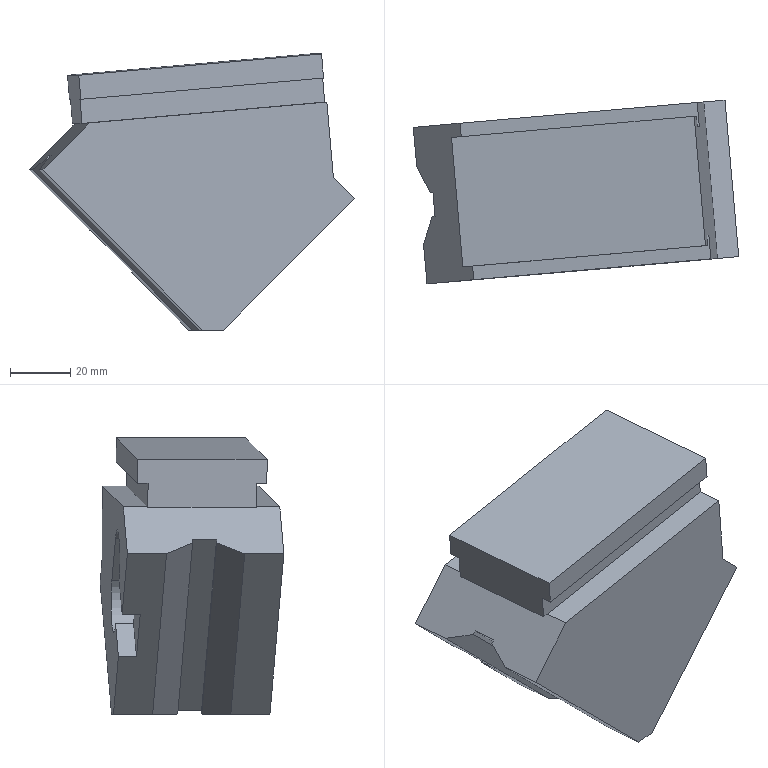Part | NX | features solid 2 | 1 solid | 35 faces | box 107.729 x 60.831 x 91.402 mm | volume 279477 mm3 | plane 33 | cylinder 2 | commonest cylinder face diameters 20 x2
STEP:
#1=CARTESIAN_POINT('',(-444.721,27.344,108.351));
#2=VERTEX_POINT('',#1);
#3=CARTESIAN_POINT('',(-445.418,35.314,108.351));
#4=VERTEX_POINT('',#3);
#5=CARTESIAN_POINT('',(-440.886,-16.489,108.351));
#6=DIRECTION('',(-0.08716,0.9962,0.));
#7=VECTOR('',#6,1000.);
#8=LINE('',#5,#7);
#9=EDGE_CURVE('',#2,#4,#8,.T.);
#10=ORIENTED_EDGE('',*,*,#9,.F.);
#11=CARTESIAN_POINT('',(-366.215,34.212,115.246));
#12=VERTEX_POINT('',#11);
#13=CARTESIAN_POINT('',(-440.646,27.701,108.709));
#14=DIRECTION('',(0.9924,0.08682,0.08716));
#15=VECTOR('',#14,1000.);
#16=LINE('',#13,#15);
#17=EDGE_CURVE('',#2,#12,#16,.T.);
#18=ORIENTED_EDGE('',*,*,#17,.T.);
#19=CARTESIAN_POINT('',(-366.913,42.182,115.246));
#20=VERTEX_POINT('',#19);
#21=CARTESIAN_POINT('',(-362.38,-9.62,115.246));
#22=DIRECTION('',(-0.08716,0.9962,0.));
#23=VECTOR('',#22,1000.);
#24=LINE('',#21,#23);
#25=EDGE_CURVE('',#12,#20,#24,.T.);
#26=ORIENTED_EDGE('',*,*,#25,.T.);
#27=CARTESIAN_POINT('',(-445.418,35.314,108.351));
#28=DIRECTION('',(0.9924,0.08682,0.08716));
#29=VECTOR('',#28,1000.);
#30=LINE('',#27,#29);
#31=EDGE_CURVE('',#4,#20,#30,.T.);
#32=ORIENTED_EDGE('',*,*,#31,.F.);
#33=EDGE_LOOP('',(#10,#18,#26,#32));
#34=FACE_BOUND('',#33,.T.);
#35=CARTESIAN_POINT('',(-440.886,-16.489,108.351));
#36=DIRECTION('',(-0.08682,-0.007596,0.9962));
#37=DIRECTION('',(0.9924,0.08682,0.08716));
#38=AXIS2_PLACEMENT_3D('',#35,#36,#37);
#39=PLANE('',#38);
#40=ADVANCED_FACE('',(#34),#39,.T.);
#41=CARTESIAN_POINT('',(-415.583,31.901,69.751));
#42=VERTEX_POINT('',#41);
#43=CARTESIAN_POINT('',(-415.06,25.924,69.751));
#44=VERTEX_POINT('',#43);
#45=CARTESIAN_POINT('',(-415.06,25.924,69.751));
#46=DIRECTION('',(0.08716,-0.9962,0.));
#47=VECTOR('',#46,1000.);
#48=LINE('',#45,#47);
#49=EDGE_CURVE('',#42,#44,#48,.T.);
#50=ORIENTED_EDGE('',*,*,#49,.F.);
#51=CARTESIAN_POINT('',(-429.629,30.672,83.85));
#52=VERTEX_POINT('',#51);
#53=CARTESIAN_POINT('',(-415.541,31.905,69.708));
#54=DIRECTION('',(-0.7044,-0.06163,0.7071));
#55=VECTOR('',#54,1000.);
#56=LINE('',#53,#55);
#57=EDGE_CURVE('',#42,#52,#56,.T.);
#58=ORIENTED_EDGE('',*,*,#57,.T.);
#59=CARTESIAN_POINT('',(-429.106,24.695,83.85));
#60=VERTEX_POINT('',#59);
#61=CARTESIAN_POINT('',(-429.106,24.695,83.85));
#62=DIRECTION('',(-0.08716,0.9962,0.));
#63=VECTOR('',#62,1000.);
#64=LINE('',#61,#63);
#65=EDGE_CURVE('',#60,#52,#64,.T.);
#66=ORIENTED_EDGE('',*,*,#65,.F.);
#67=CARTESIAN_POINT('',(-415.018,25.927,69.708));
#68=DIRECTION('',(-0.7044,-0.06163,0.7071));
#69=VECTOR('',#68,1000.);
#70=LINE('',#67,#69);
#71=EDGE_CURVE('',#44,#60,#70,.T.);
#72=ORIENTED_EDGE('',*,*,#71,.F.);
#73=EDGE_LOOP('',(#50,#58,#66,#72));
#74=FACE_BOUND('',#73,.T.);
#75=CARTESIAN_POINT('',(-415.018,25.927,69.708));
#76=DIRECTION('',(-0.7044,-0.06163,-0.7071));
#77=DIRECTION('',(-0.7044,-0.06163,0.7071));
#78=AXIS2_PLACEMENT_3D('',#75,#76,#77);
#79=PLANE('',#78);
#80=ADVANCED_FACE('',(#74),#79,.F.);
#81=CARTESIAN_POINT('',(-402.018,39.111,83.893));
#82=VERTEX_POINT('',#81);
#83=CARTESIAN_POINT('',(-416.064,37.882,97.992));
#84=VERTEX_POINT('',#83);
#85=CARTESIAN_POINT('',(-401.976,39.114,83.85));
#86=DIRECTION('',(-0.7044,-0.06163,0.7071));
#87=VECTOR('',#86,1000.);
#88=LINE('',#85,#87);
#89=EDGE_CURVE('',#82,#84,#88,.T.);
#90=ORIENTED_EDGE('',*,*,#89,.F.);
#91=CARTESIAN_POINT('',(-400.972,27.156,83.893));
#92=VERTEX_POINT('',#91);
#93=CARTESIAN_POINT('',(-400.972,27.156,83.893));
#94=DIRECTION('',(-0.08716,0.9962,0.));
#95=VECTOR('',#94,1000.);
#96=LINE('',#93,#95);
#97=EDGE_CURVE('',#92,#82,#96,.T.);
#98=ORIENTED_EDGE('',*,*,#97,.F.);
#99=CARTESIAN_POINT('',(-415.018,25.927,97.992));
#100=VERTEX_POINT('',#99);
#101=CARTESIAN_POINT('',(-400.93,27.16,83.85));
#102=DIRECTION('',(-0.7044,-0.06163,0.7071));
#103=VECTOR('',#102,1000.);
#104=LINE('',#101,#103);
#105=EDGE_CURVE('',#92,#100,#104,.T.);
#106=ORIENTED_EDGE('',*,*,#105,.T.);
#107=CARTESIAN_POINT('',(-415.018,25.927,97.992));
#108=DIRECTION('',(-0.08716,0.9962,0.));
#109=VECTOR('',#108,1000.);
#110=LINE('',#107,#109);
#111=EDGE_CURVE('',#100,#84,#110,.T.);
#112=ORIENTED_EDGE('',*,*,#111,.T.);
#113=EDGE_LOOP('',(#90,#98,#106,#112));
#114=FACE_BOUND('',#113,.T.);
#115=CARTESIAN_POINT('',(-400.93,27.16,83.85));
#116=DIRECTION('',(-0.7044,-0.06163,-0.7071));
#117=DIRECTION('',(-0.7044,-0.06163,0.7071));
#118=AXIS2_PLACEMENT_3D('',#115,#116,#117);
#119=PLANE('',#118);
#120=ADVANCED_FACE('',(#114),#119,.T.);
#121=CARTESIAN_POINT('',(-357.698,42.988,83.27));
#122=VERTEX_POINT('',#121);
#123=CARTESIAN_POINT('',(-401.019,39.198,39.783));
#124=VERTEX_POINT('',#123);
#125=CARTESIAN_POINT('',(-357.698,42.988,83.27));
#126=DIRECTION('',(-0.7044,-0.06163,-0.7071));
#127=VECTOR('',#126,1000.);
#128=LINE('',#125,#127);
#129=EDGE_CURVE('',#122,#124,#128,.T.);
#130=ORIENTED_EDGE('',*,*,#129,.T.);
#131=CARTESIAN_POINT('',(-408.064,38.582,39.783));
#132=VERTEX_POINT('',#131);
#133=CARTESIAN_POINT('',(-401.019,39.198,39.783));
#134=DIRECTION('',(-0.9962,-0.08716,0.));
#135=VECTOR('',#134,1000.);
#136=LINE('',#133,#135);
#137=EDGE_CURVE('',#124,#132,#136,.T.);
#138=ORIENTED_EDGE('',*,*,#137,.T.);
#139=CARTESIAN_POINT('',(-426.969,36.928,58.761));
#140=VERTEX_POINT('',#139);
#141=CARTESIAN_POINT('',(-460.895,33.96,92.816));
#142=DIRECTION('',(0.7044,0.06163,-0.7071));
#143=VECTOR('',#142,1000.);
#144=LINE('',#141,#143);
#145=EDGE_CURVE('',#140,#132,#144,.T.);
#146=ORIENTED_EDGE('',*,*,#145,.F.);
#147=CARTESIAN_POINT('',(-416.064,37.882,69.708));
#148=VERTEX_POINT('',#147);
#149=CARTESIAN_POINT('',(-401.976,39.114,83.85));
#150=DIRECTION('',(-0.7044,-0.06163,-0.7071));
#151=VECTOR('',#150,1000.);
#152=LINE('',#149,#151);
#153=EDGE_CURVE('',#148,#140,#152,.T.);
#154=ORIENTED_EDGE('',*,*,#153,.F.);
#155=CARTESIAN_POINT('',(-416.106,37.878,69.751));
#156=VERTEX_POINT('',#155);
#157=CARTESIAN_POINT('',(-416.106,37.878,69.751));
#158=DIRECTION('',(0.7044,0.06163,-0.7071));
#159=VECTOR('',#158,1000.);
#160=LINE('',#157,#159);
#161=EDGE_CURVE('',#156,#148,#160,.T.);
#162=ORIENTED_EDGE('',*,*,#161,.F.);
#163=CARTESIAN_POINT('',(-409.062,38.494,76.822));
#164=DIRECTION('',(0.08716,-0.9962,0.));
#165=DIRECTION('',(0.9029,0.07899,-0.4226));
#166=AXIS2_PLACEMENT_3D('',#163,#164,#165);
#167=CIRCLE('',#166,10.);
#168=EDGE_CURVE('',#156,#82,#167,.T.);
#169=ORIENTED_EDGE('',*,*,#168,.T.);
#170=ORIENTED_EDGE('',*,*,#89,.T.);
#171=CARTESIAN_POINT('',(-430.152,36.649,83.85));
#172=VERTEX_POINT('',#171);
#173=CARTESIAN_POINT('',(-423.108,37.266,90.921));
#174=DIRECTION('',(0.08716,-0.9962,0.));
#175=DIRECTION('',(0.9029,0.07899,-0.4226));
#176=AXIS2_PLACEMENT_3D('',#173,#174,#175);
#177=CIRCLE('',#176,10.);
#178=EDGE_CURVE('',#84,#172,#177,.T.);
#179=ORIENTED_EDGE('',*,*,#178,.T.);
#180=CARTESIAN_POINT('',(-441.058,35.695,72.903));
#181=VERTEX_POINT('',#180);
#182=CARTESIAN_POINT('',(-416.064,37.882,97.992));
#183=DIRECTION('',(-0.7044,-0.06163,-0.7071));
#184=VECTOR('',#183,1000.);
#185=LINE('',#182,#184);
#186=EDGE_CURVE('',#172,#181,#185,.T.);
#187=ORIENTED_EDGE('',*,*,#186,.T.);
#188=CARTESIAN_POINT('',(-460.895,33.96,92.816));
#189=VERTEX_POINT('',#188);
#190=CARTESIAN_POINT('',(-460.895,33.96,92.816));
#191=DIRECTION('',(0.7044,0.06163,-0.7071));
#192=VECTOR('',#191,1000.);
#193=LINE('',#190,#192);
#194=EDGE_CURVE('',#189,#181,#193,.T.);
#195=ORIENTED_EDGE('',*,*,#194,.F.);
#196=CARTESIAN_POINT('',(-445.418,35.314,108.351));
#197=DIRECTION('',(-0.7044,-0.06163,-0.7071));
#198=VECTOR('',#197,1000.);
#199=LINE('',#196,#198);
#200=EDGE_CURVE('',#4,#189,#199,.T.);
#201=ORIENTED_EDGE('',*,*,#200,.F.);
#202=ORIENTED_EDGE('',*,*,#31,.T.);
#203=CARTESIAN_POINT('',(-364.742,42.372,90.341));
#204=VERTEX_POINT('',#203);
#205=CARTESIAN_POINT('',(-366.913,42.182,115.246));
#206=DIRECTION('',(0.08682,0.007596,-0.9962));
#207=VECTOR('',#206,1000.);
#208=LINE('',#205,#207);
#209=EDGE_CURVE('',#20,#204,#208,.T.);
#210=ORIENTED_EDGE('',*,*,#209,.T.);
#211=CARTESIAN_POINT('',(-364.742,42.372,90.341));
#212=DIRECTION('',(0.7044,0.06163,-0.7071));
#213=VECTOR('',#212,1000.);
#214=LINE('',#211,#213);
#215=EDGE_CURVE('',#204,#122,#214,.T.);
#216=ORIENTED_EDGE('',*,*,#215,.T.);
#217=EDGE_LOOP('',(#130,#138,#146,#154,#162,#169,#170,#179,#187,#195,#201,#202,#210,#216));
#218=FACE_BOUND('',#217,.T.);
#219=CARTESIAN_POINT('',(-460.895,33.96,92.816));
#220=DIRECTION('',(0.08716,-0.9962,0.));
#221=DIRECTION('',(0.,0.,-1.));
#222=AXIS2_PLACEMENT_3D('',#219,#220,#221);
#223=PLANE('',#222);
#224=ADVANCED_FACE('',(#218),#223,.F.);
#225=ORIENTED_EDGE('',*,*,#145,.T.);
#226=CARTESIAN_POINT('',(-406.93,25.622,39.783));
#227=VERTEX_POINT('',#226);
#228=CARTESIAN_POINT('',(-406.93,25.622,39.783));
#229=DIRECTION('',(0.08716,-0.9962,0.));
#230=VECTOR('',#229,1000.);
#231=LINE('',#228,#230);
#232=EDGE_CURVE('',#132,#227,#231,.T.);
#233=ORIENTED_EDGE('',*,*,#232,.T.);
#234=CARTESIAN_POINT('',(-459.761,20.999,92.816));
#235=VERTEX_POINT('',#234);
#236=CARTESIAN_POINT('',(-459.761,20.999,92.816));
#237=DIRECTION('',(-0.7044,-0.06163,0.7071));
#238=VECTOR('',#237,1000.);
#239=LINE('',#236,#238);
#240=EDGE_CURVE('',#227,#235,#239,.T.);
#241=ORIENTED_EDGE('',*,*,#240,.T.);
#242=CARTESIAN_POINT('',(-456.363,-17.843,92.816));
#243=DIRECTION('',(-0.08716,0.9962,0.));
#244=VECTOR('',#243,1000.);
#245=LINE('',#242,#244);
#246=EDGE_CURVE('',#235,#189,#245,.T.);
#247=ORIENTED_EDGE('',*,*,#246,.T.);
#248=ORIENTED_EDGE('',*,*,#194,.T.);
#249=CARTESIAN_POINT('',(-440.535,29.718,72.903));
#250=VERTEX_POINT('',#249);
#251=CARTESIAN_POINT('',(-436.526,-16.107,72.903));
#252=DIRECTION('',(-0.08716,0.9962,0.));
#253=VECTOR('',#252,1000.);
#254=LINE('',#251,#253);
#255=EDGE_CURVE('',#250,#181,#254,.T.);
#256=ORIENTED_EDGE('',*,*,#255,.F.);
#257=CARTESIAN_POINT('',(-426.446,30.951,58.761));
#258=VERTEX_POINT('',#257);
#259=CARTESIAN_POINT('',(-460.372,27.982,92.816));
#260=DIRECTION('',(-0.7044,-0.06163,0.7071));
#261=VECTOR('',#260,1000.);
#262=LINE('',#259,#261);
#263=EDGE_CURVE('',#258,#250,#262,.T.);
#264=ORIENTED_EDGE('',*,*,#263,.F.);
#265=CARTESIAN_POINT('',(-422.437,-14.874,58.761));
#266=DIRECTION('',(-0.08716,0.9962,0.));
#267=VECTOR('',#266,1000.);
#268=LINE('',#265,#267);
#269=EDGE_CURVE('',#258,#140,#268,.T.);
#270=ORIENTED_EDGE('',*,*,#269,.T.);
#271=EDGE_LOOP('',(#225,#233,#241,#247,#248,#256,#264,#270));
#272=FACE_BOUND('',#271,.T.);
#273=CARTESIAN_POINT('',(-456.363,-17.843,92.816));
#274=DIRECTION('',(0.7044,0.06163,0.7071));
#275=DIRECTION('',(0.7044,0.06163,-0.7071));
#276=AXIS2_PLACEMENT_3D('',#273,#274,#275);
#277=PLANE('',#276);
#278=ADVANCED_FACE('',(#272),#277,.F.);
#279=CARTESIAN_POINT('',(-457.497,-4.882,92.816));
#280=VERTEX_POINT('',#279);
#281=CARTESIAN_POINT('',(-404.665,-0.2603,39.783));
#282=VERTEX_POINT('',#281);
#283=CARTESIAN_POINT('',(-457.497,-4.882,92.816));
#284=DIRECTION('',(0.7044,0.06163,-0.7071));
#285=VECTOR('',#284,1000.);
#286=LINE('',#283,#285);
#287=EDGE_CURVE('',#280,#282,#286,.T.);
#288=ORIENTED_EDGE('',*,*,#287,.T.);
#289=CARTESIAN_POINT('',(-403.531,-13.22,39.783));
#290=VERTEX_POINT('',#289);
#291=CARTESIAN_POINT('',(-403.531,-13.22,39.783));
#292=DIRECTION('',(0.08716,-0.9962,0.));
#293=VECTOR('',#292,1000.);
#294=LINE('',#291,#293);
#295=EDGE_CURVE('',#282,#290,#294,.T.);
#296=ORIENTED_EDGE('',*,*,#295,.T.);
#297=CARTESIAN_POINT('',(-456.363,-17.843,92.816));
#298=VERTEX_POINT('',#297);
#299=CARTESIAN_POINT('',(-456.363,-17.843,92.816));
#300=DIRECTION('',(0.7044,0.06163,-0.7071));
#301=VECTOR('',#300,1000.);
#302=LINE('',#299,#301);
#303=EDGE_CURVE('',#298,#290,#302,.T.);
#304=ORIENTED_EDGE('',*,*,#303,.F.);
#305=CARTESIAN_POINT('',(-456.363,-17.843,92.816));
#306=DIRECTION('',(-0.08716,0.9962,0.));
#307=VECTOR('',#306,1000.);
#308=LINE('',#305,#307);
#309=EDGE_CURVE('',#298,#280,#308,.T.);
#310=ORIENTED_EDGE('',*,*,#309,.T.);
#311=EDGE_LOOP('',(#288,#296,#304,#310));
#312=FACE_BOUND('',#311,.T.);
#313=CARTESIAN_POINT('',(-456.363,-17.843,92.816));
#314=DIRECTION('',(0.7044,0.06163,0.7071));
#315=DIRECTION('',(0.7044,0.06163,-0.7071));
#316=AXIS2_PLACEMENT_3D('',#313,#314,#315);
#317=PLANE('',#316);
#318=ADVANCED_FACE('',(#312),#317,.F.);
#319=CARTESIAN_POINT('',(-453.701,4.474,97.412));
#320=VERTEX_POINT('',#319);
#321=CARTESIAN_POINT('',(-454.624,4.394,96.486));
#322=VERTEX_POINT('',#321);
#323=CARTESIAN_POINT('',(-453.701,4.474,97.412));
#324=DIRECTION('',(-0.7044,-0.06163,-0.7071));
#325=VECTOR('',#324,1000.);
#326=LINE('',#323,#325);
#327=EDGE_CURVE('',#320,#322,#326,.T.);
#328=ORIENTED_EDGE('',*,*,#327,.T.);
#329=CARTESIAN_POINT('',(-457.497,-4.882,92.816));
#330=DIRECTION('',(0.2767,0.8935,0.3536));
#331=VECTOR('',#330,1000.);
#332=LINE('',#329,#331);
#333=EDGE_CURVE('',#280,#322,#332,.T.);
#334=ORIENTED_EDGE('',*,*,#333,.F.);
#335=ORIENTED_EDGE('',*,*,#309,.F.);
#336=CARTESIAN_POINT('',(-440.886,-16.489,108.351));
#337=VERTEX_POINT('',#336);
#338=CARTESIAN_POINT('',(-440.886,-16.489,108.351));
#339=DIRECTION('',(-0.7044,-0.06163,-0.7071));
#340=VECTOR('',#339,1000.);
#341=LINE('',#338,#340);
#342=EDGE_CURVE('',#337,#298,#341,.T.);
#343=ORIENTED_EDGE('',*,*,#342,.F.);
#344=CARTESIAN_POINT('',(-441.584,-8.519,108.351));
#345=VERTEX_POINT('',#344);
#346=CARTESIAN_POINT('',(-440.886,-16.489,108.351));
#347=DIRECTION('',(-0.08716,0.9962,0.));
#348=VECTOR('',#347,1000.);
#349=LINE('',#346,#348);
#350=EDGE_CURVE('',#337,#345,#349,.T.);
#351=ORIENTED_EDGE('',*,*,#350,.T.);
#352=CARTESIAN_POINT('',(-440.886,-16.489,108.351));
#353=DIRECTION('',(-0.08716,0.9962,0.));
#354=VECTOR('',#353,1000.);
#355=LINE('',#352,#354);
#356=EDGE_CURVE('',#345,#2,#355,.T.);
#357=ORIENTED_EDGE('',*,*,#356,.T.);
#358=ORIENTED_EDGE('',*,*,#9,.T.);
#359=ORIENTED_EDGE('',*,*,#200,.T.);
#360=ORIENTED_EDGE('',*,*,#246,.F.);
#361=CARTESIAN_POINT('',(-455.321,12.363,96.486));
#362=VERTEX_POINT('',#361);
#363=CARTESIAN_POINT('',(-459.761,20.999,92.816));
#364=DIRECTION('',(-0.4277,0.8319,-0.3536));
#365=VECTOR('',#364,1000.);
#366=LINE('',#363,#365);
#367=EDGE_CURVE('',#362,#235,#366,.T.);
#368=ORIENTED_EDGE('',*,*,#367,.F.);
#369=CARTESIAN_POINT('',(-454.399,12.444,97.412));
#370=VERTEX_POINT('',#369);
#371=CARTESIAN_POINT('',(-454.399,12.444,97.412));
#372=DIRECTION('',(-0.7044,-0.06163,-0.7071));
#373=VECTOR('',#372,1000.);
#374=LINE('',#371,#373);
#375=EDGE_CURVE('',#370,#362,#374,.T.);
#376=ORIENTED_EDGE('',*,*,#375,.F.);
#377=CARTESIAN_POINT('',(-453.701,4.474,97.412));
#378=DIRECTION('',(-0.08716,0.9962,0.));
#379=VECTOR('',#378,1000.);
#380=LINE('',#377,#379);
#381=EDGE_CURVE('',#320,#370,#380,.T.);
#382=ORIENTED_EDGE('',*,*,#381,.F.);
#383=EDGE_LOOP('',(#328,#334,#335,#343,#351,#357,#358,#359,#360,#368,#376,#382));
#384=FACE_BOUND('',#383,.T.);
#385=CARTESIAN_POINT('',(-440.886,-16.489,108.351));
#386=DIRECTION('',(0.7044,0.06163,-0.7071));
#387=DIRECTION('',(-0.7044,-0.06163,-0.7071));
#388=AXIS2_PLACEMENT_3D('',#385,#386,#387);
#389=PLANE('',#388);
#390=ADVANCED_FACE('',(#384),#389,.F.);
#391=CARTESIAN_POINT('',(-398.968,17.293,39.918));
#392=VERTEX_POINT('',#391);
#393=CARTESIAN_POINT('',(-399.131,17.611,39.783));
#394=VERTEX_POINT('',#393);
#395=CARTESIAN_POINT('',(-398.968,17.293,39.918));
#396=DIRECTION('',(-0.4277,0.8319,-0.3536));
#397=VECTOR('',#396,1000.);
#398=LINE('',#395,#397);
#399=EDGE_CURVE('',#392,#394,#398,.T.);
#400=ORIENTED_EDGE('',*,*,#399,.T.);
#401=CARTESIAN_POINT('',(-401.019,39.198,39.783));
#402=DIRECTION('',(-0.08716,0.9962,0.));
#403=VECTOR('',#402,1000.);
#404=LINE('',#401,#403);
#405=EDGE_CURVE('',#394,#124,#404,.T.);
#406=ORIENTED_EDGE('',*,*,#405,.T.);
#407=ORIENTED_EDGE('',*,*,#129,.F.);
#408=CARTESIAN_POINT('',(-353.166,-8.814,83.27));
#409=VERTEX_POINT('',#408);
#410=CARTESIAN_POINT('',(-353.166,-8.814,83.27));
#411=DIRECTION('',(-0.08716,0.9962,0.));
#412=VECTOR('',#411,1000.);
#413=LINE('',#410,#412);
#414=EDGE_CURVE('',#409,#122,#413,.T.);
#415=ORIENTED_EDGE('',*,*,#414,.F.);
#416=CARTESIAN_POINT('',(-396.487,-12.604,39.783));
#417=VERTEX_POINT('',#416);
#418=CARTESIAN_POINT('',(-353.166,-8.814,83.27));
#419=DIRECTION('',(-0.7044,-0.06163,-0.7071));
#420=VECTOR('',#419,1000.);
#421=LINE('',#418,#420);
#422=EDGE_CURVE('',#409,#417,#421,.T.);
#423=ORIENTED_EDGE('',*,*,#422,.T.);
#424=CARTESIAN_POINT('',(-398.376,8.983,39.783));
#425=VERTEX_POINT('',#424);
#426=CARTESIAN_POINT('',(-397.621,0.356,39.783));
#427=DIRECTION('',(-0.08716,0.9962,0.));
#428=VECTOR('',#427,1000.);
#429=LINE('',#426,#428);
#430=EDGE_CURVE('',#417,#425,#429,.T.);
#431=ORIENTED_EDGE('',*,*,#430,.T.);
#432=CARTESIAN_POINT('',(-398.27,9.324,39.918));
#433=VERTEX_POINT('',#432);
#434=CARTESIAN_POINT('',(-405.017,-12.462,31.298));
#435=DIRECTION('',(0.2767,0.8935,0.3536));
#436=VECTOR('',#435,1000.);
#437=LINE('',#434,#436);
#438=EDGE_CURVE('',#425,#433,#437,.T.);
#439=ORIENTED_EDGE('',*,*,#438,.T.);
#440=CARTESIAN_POINT('',(-397.348,9.405,40.844));
#441=VERTEX_POINT('',#440);
#442=CARTESIAN_POINT('',(-397.348,9.405,40.844));
#443=DIRECTION('',(-0.7044,-0.06163,-0.7071));
#444=VECTOR('',#443,1000.);
#445=LINE('',#442,#444);
#446=EDGE_CURVE('',#441,#433,#445,.T.);
#447=ORIENTED_EDGE('',*,*,#446,.F.);
#448=CARTESIAN_POINT('',(-398.045,17.374,40.844));
#449=VERTEX_POINT('',#448);
#450=CARTESIAN_POINT('',(-397.348,9.405,40.844));
#451=DIRECTION('',(-0.08716,0.9962,0.));
#452=VECTOR('',#451,1000.);
#453=LINE('',#450,#452);
#454=EDGE_CURVE('',#441,#449,#453,.T.);
#455=ORIENTED_EDGE('',*,*,#454,.T.);
#456=CARTESIAN_POINT('',(-398.045,17.374,40.844));
#457=DIRECTION('',(-0.7044,-0.06163,-0.7071));
#458=VECTOR('',#457,1000.);
#459=LINE('',#456,#458);
#460=EDGE_CURVE('',#449,#392,#459,.T.);
#461=ORIENTED_EDGE('',*,*,#460,.T.);
#462=EDGE_LOOP('',(#400,#406,#407,#415,#423,#431,#439,#447,#455,#461));
#463=FACE_BOUND('',#462,.T.);
#464=CARTESIAN_POINT('',(-353.166,-8.814,83.27));
#465=DIRECTION('',(0.7044,0.06163,-0.7071));
#466=DIRECTION('',(-0.7044,-0.06163,-0.7071));
#467=AXIS2_PLACEMENT_3D('',#464,#465,#466);
#468=PLANE('',#467);
#469=ADVANCED_FACE('',(#463),#468,.T.);
#470=ORIENTED_EDGE('',*,*,#215,.F.);
#471=CARTESIAN_POINT('',(-360.21,-9.43,90.341));
#472=VERTEX_POINT('',#471);
#473=CARTESIAN_POINT('',(-360.21,-9.43,90.341));
#474=DIRECTION('',(-0.08716,0.9962,0.));
#475=VECTOR('',#474,1000.);
#476=LINE('',#473,#475);
#477=EDGE_CURVE('',#472,#204,#476,.T.);
#478=ORIENTED_EDGE('',*,*,#477,.F.);
#479=CARTESIAN_POINT('',(-360.21,-9.43,90.341));
#480=DIRECTION('',(0.7044,0.06163,-0.7071));
#481=VECTOR('',#480,1000.);
#482=LINE('',#479,#481);
#483=EDGE_CURVE('',#472,#409,#482,.T.);
#484=ORIENTED_EDGE('',*,*,#483,.T.);
#485=ORIENTED_EDGE('',*,*,#414,.T.);
#486=EDGE_LOOP('',(#470,#478,#484,#485));
#487=FACE_BOUND('',#486,.T.);
#488=CARTESIAN_POINT('',(-360.21,-9.43,90.341));
#489=DIRECTION('',(0.7044,0.06163,0.7071));
#490=DIRECTION('',(0.7044,0.06163,-0.7071));
#491=AXIS2_PLACEMENT_3D('',#488,#489,#490);
#492=PLANE('',#491);
#493=ADVANCED_FACE('',(#487),#492,.T.);
#494=ORIENTED_EDGE('',*,*,#209,.F.);
#495=ORIENTED_EDGE('',*,*,#25,.F.);
#496=CARTESIAN_POINT('',(-366.91,34.152,123.215));
#497=VERTEX_POINT('',#496);
#498=CARTESIAN_POINT('',(-366.91,34.152,123.215));
#499=DIRECTION('',(0.08682,0.007596,-0.9962));
#500=VECTOR('',#499,1000.);
#501=LINE('',#498,#500);
#502=EDGE_CURVE('',#497,#12,#501,.T.);
#503=ORIENTED_EDGE('',*,*,#502,.F.);
#504=CARTESIAN_POINT('',(-367.215,37.638,123.215));
#505=VERTEX_POINT('',#504);
#506=CARTESIAN_POINT('',(-367.215,37.638,123.215));
#507=DIRECTION('',(0.08716,-0.9962,0.));
#508=VECTOR('',#507,1000.);
#509=LINE('',#506,#508);
#510=EDGE_CURVE('',#505,#497,#509,.T.);
#511=ORIENTED_EDGE('',*,*,#510,.F.);
#512=CARTESIAN_POINT('',(-367.91,37.578,131.185));
#513=VERTEX_POINT('',#512);
#514=CARTESIAN_POINT('',(-367.91,37.578,131.185));
#515=DIRECTION('',(0.08682,0.007596,-0.9962));
#516=VECTOR('',#515,1000.);
#517=LINE('',#514,#516);
#518=EDGE_CURVE('',#513,#505,#517,.T.);
#519=ORIENTED_EDGE('',*,*,#518,.F.);
#520=CARTESIAN_POINT('',(-364.162,-5.259,131.185));
#521=VERTEX_POINT('',#520);
#522=CARTESIAN_POINT('',(-367.91,37.578,131.185));
#523=DIRECTION('',(0.08716,-0.9962,0.));
#524=VECTOR('',#523,1000.);
#525=LINE('',#522,#524);
#526=EDGE_CURVE('',#513,#521,#525,.T.);
#527=ORIENTED_EDGE('',*,*,#526,.T.);
#528=CARTESIAN_POINT('',(-363.467,-5.198,123.215));
#529=VERTEX_POINT('',#528);
#530=CARTESIAN_POINT('',(-364.162,-5.259,131.185));
#531=DIRECTION('',(0.08682,0.007596,-0.9962));
#532=VECTOR('',#531,1000.);
#533=LINE('',#530,#532);
#534=EDGE_CURVE('',#521,#529,#533,.T.);
#535=ORIENTED_EDGE('',*,*,#534,.T.);
#536=CARTESIAN_POINT('',(-363.772,-1.711,123.215));
#537=VERTEX_POINT('',#536);
#538=CARTESIAN_POINT('',(-367.215,37.638,123.215));
#539=DIRECTION('',(0.08716,-0.9962,0.));
#540=VECTOR('',#539,1000.);
#541=LINE('',#538,#540);
#542=EDGE_CURVE('',#537,#529,#541,.T.);
#543=ORIENTED_EDGE('',*,*,#542,.F.);
#544=CARTESIAN_POINT('',(-363.078,-1.651,115.246));
#545=VERTEX_POINT('',#544);
#546=CARTESIAN_POINT('',(-363.772,-1.711,123.215));
#547=DIRECTION('',(0.08682,0.007596,-0.9962));
#548=VECTOR('',#547,1000.);
#549=LINE('',#546,#548);
#550=EDGE_CURVE('',#537,#545,#549,.T.);
#551=ORIENTED_EDGE('',*,*,#550,.T.);
#552=CARTESIAN_POINT('',(-362.38,-9.62,115.246));
#553=VERTEX_POINT('',#552);
#554=CARTESIAN_POINT('',(-362.38,-9.62,115.246));
#555=DIRECTION('',(-0.08716,0.9962,0.));
#556=VECTOR('',#555,1000.);
#557=LINE('',#554,#556);
#558=EDGE_CURVE('',#553,#545,#557,.T.);
#559=ORIENTED_EDGE('',*,*,#558,.F.);
#560=CARTESIAN_POINT('',(-362.38,-9.62,115.246));
#561=DIRECTION('',(0.08682,0.007596,-0.9962));
#562=VECTOR('',#561,1000.);
#563=LINE('',#560,#562);
#564=EDGE_CURVE('',#553,#472,#563,.T.);
#565=ORIENTED_EDGE('',*,*,#564,.T.);
#566=ORIENTED_EDGE('',*,*,#477,.T.);
#567=EDGE_LOOP('',(#494,#495,#503,#511,#519,#527,#535,#543,#551,#559,#565,#566));
#568=FACE_BOUND('',#567,.T.);
#569=CARTESIAN_POINT('',(-362.38,-9.62,115.246));
#570=DIRECTION('',(0.9924,0.08682,0.08716));
#571=DIRECTION('',(0.08682,0.007596,-0.9962));
#572=AXIS2_PLACEMENT_3D('',#569,#570,#571);
#573=PLANE('',#572);
#574=ADVANCED_FACE('',(#568),#573,.T.);
#575=CARTESIAN_POINT('',(-437.508,-8.162,108.709));
#576=DIRECTION('',(0.9924,0.08682,0.08716));
#577=VECTOR('',#576,1000.);
#578=LINE('',#575,#577);
#579=EDGE_CURVE('',#345,#545,#578,.T.);
#580=ORIENTED_EDGE('',*,*,#579,.F.);
#581=ORIENTED_EDGE('',*,*,#350,.F.);
#582=CARTESIAN_POINT('',(-440.886,-16.489,108.351));
#583=DIRECTION('',(0.9924,0.08682,0.08716));
#584=VECTOR('',#583,1000.);
#585=LINE('',#582,#584);
#586=EDGE_CURVE('',#337,#553,#585,.T.);
#587=ORIENTED_EDGE('',*,*,#586,.T.);
#588=ORIENTED_EDGE('',*,*,#558,.T.);
#589=EDGE_LOOP('',(#580,#581,#587,#588));
#590=FACE_BOUND('',#589,.T.);
#591=CARTESIAN_POINT('',(-440.886,-16.489,108.351));
#592=DIRECTION('',(-0.08682,-0.007596,0.9962));
#593=DIRECTION('',(0.9924,0.08682,0.08716));
#594=AXIS2_PLACEMENT_3D('',#591,#592,#593);
#595=PLANE('',#594);
#596=ADVANCED_FACE('',(#590),#595,.T.);
#597=ORIENTED_EDGE('',*,*,#303,.T.);
#598=CARTESIAN_POINT('',(-456.363,-17.843,39.783));
#599=DIRECTION('',(0.9962,0.08716,0.));
#600=VECTOR('',#599,1000.);
#601=LINE('',#598,#600);
#602=EDGE_CURVE('',#290,#417,#601,.T.);
#603=ORIENTED_EDGE('',*,*,#602,.T.);
#604=ORIENTED_EDGE('',*,*,#422,.F.);
#605=ORIENTED_EDGE('',*,*,#483,.F.);
#606=ORIENTED_EDGE('',*,*,#564,.F.);
#607=ORIENTED_EDGE('',*,*,#586,.F.);
#608=ORIENTED_EDGE('',*,*,#342,.T.);
#609=EDGE_LOOP('',(#597,#603,#604,#605,#606,#607,#608));
#610=FACE_BOUND('',#609,.T.);
#611=CARTESIAN_POINT('',(-456.363,-17.843,92.816));
#612=DIRECTION('',(0.08716,-0.9962,0.));
#613=DIRECTION('',(0.,0.,-1.));
#614=AXIS2_PLACEMENT_3D('',#611,#612,#613);
#615=PLANE('',#614);
#616=ADVANCED_FACE('',(#610),#615,.T.);
#617=ORIENTED_EDGE('',*,*,#438,.F.);
#618=CARTESIAN_POINT('',(-407.818,-4.894,39.783));
#619=DIRECTION('',(-0.5625,-0.8268,0.));
#620=VECTOR('',#619,1000.);
#621=LINE('',#618,#620);
#622=EDGE_CURVE('',#425,#282,#621,.T.);
#623=ORIENTED_EDGE('',*,*,#622,.T.);
#624=ORIENTED_EDGE('',*,*,#287,.F.);
#625=ORIENTED_EDGE('',*,*,#333,.T.);
#626=CARTESIAN_POINT('',(-398.27,9.324,39.918));
#627=DIRECTION('',(-0.7044,-0.06163,0.7071));
#628=VECTOR('',#627,1000.);
#629=LINE('',#626,#628);
#630=EDGE_CURVE('',#433,#322,#629,.T.);
#631=ORIENTED_EDGE('',*,*,#630,.F.);
#632=EDGE_LOOP('',(#617,#623,#624,#625,#631));
#633=FACE_BOUND('',#632,.T.);
#634=CARTESIAN_POINT('',(-401.143,0.04786,36.247));
#635=DIRECTION('',(0.6536,-0.4447,0.6124));
#636=DIRECTION('',(0.7044,0.06163,-0.7071));
#637=AXIS2_PLACEMENT_3D('',#634,#635,#636);
#638=PLANE('',#637);
#639=ADVANCED_FACE('',(#633),#638,.F.);
#640=ORIENTED_EDGE('',*,*,#240,.F.);
#641=CARTESIAN_POINT('',(-382.743,0.7768,39.783));
#642=DIRECTION('',(0.6976,-0.7165,0.));
#643=VECTOR('',#642,1000.);
#644=LINE('',#641,#643);
#645=EDGE_CURVE('',#227,#394,#644,.T.);
#646=ORIENTED_EDGE('',*,*,#645,.T.);
#647=ORIENTED_EDGE('',*,*,#399,.F.);
#648=CARTESIAN_POINT('',(-398.968,17.293,39.918));
#649=DIRECTION('',(-0.7044,-0.06163,0.7071));
#650=VECTOR('',#649,1000.);
#651=LINE('',#648,#650);
#652=EDGE_CURVE('',#392,#362,#651,.T.);
#653=ORIENTED_EDGE('',*,*,#652,.T.);
#654=ORIENTED_EDGE('',*,*,#367,.T.);
#655=EDGE_LOOP('',(#640,#646,#647,#653,#654));
#656=FACE_BOUND('',#655,.T.);
#657=CARTESIAN_POINT('',(-403.408,25.93,36.247));
#658=DIRECTION('',(0.5665,0.5515,0.6124));
#659=DIRECTION('',(0.7044,0.06163,-0.7071));
#660=AXIS2_PLACEMENT_3D('',#657,#658,#659);
#661=PLANE('',#660);
#662=ADVANCED_FACE('',(#656),#661,.F.);
#663=ORIENTED_EDGE('',*,*,#375,.T.);
#664=ORIENTED_EDGE('',*,*,#652,.F.);
#665=ORIENTED_EDGE('',*,*,#460,.F.);
#666=CARTESIAN_POINT('',(-398.045,17.374,40.844));
#667=DIRECTION('',(-0.7044,-0.06163,0.7071));
#668=VECTOR('',#667,1000.);
#669=LINE('',#666,#668);
#670=EDGE_CURVE('',#449,#370,#669,.T.);
#671=ORIENTED_EDGE('',*,*,#670,.T.);
#672=EDGE_LOOP('',(#663,#664,#665,#671));
#673=FACE_BOUND('',#672,.T.);
#674=CARTESIAN_POINT('',(-398.045,17.374,40.844));
#675=DIRECTION('',(-0.08716,0.9962,0.));
#676=DIRECTION('',(0.,0.,1.));
#677=AXIS2_PLACEMENT_3D('',#674,#675,#676);
#678=PLANE('',#677);
#679=ADVANCED_FACE('',(#673),#678,.F.);
#680=ORIENTED_EDGE('',*,*,#381,.T.);
#681=ORIENTED_EDGE('',*,*,#670,.F.);
#682=ORIENTED_EDGE('',*,*,#454,.F.);
#683=CARTESIAN_POINT('',(-397.348,9.405,40.844));
#684=DIRECTION('',(-0.7044,-0.06163,0.7071));
#685=VECTOR('',#684,1000.);
#686=LINE('',#683,#685);
#687=EDGE_CURVE('',#441,#320,#686,.T.);
#688=ORIENTED_EDGE('',*,*,#687,.T.);
#689=EDGE_LOOP('',(#680,#681,#682,#688));
#690=FACE_BOUND('',#689,.T.);
#691=CARTESIAN_POINT('',(-397.348,9.405,40.844));
#692=DIRECTION('',(0.7044,0.06163,0.7071));
#693=DIRECTION('',(0.7044,0.06163,-0.7071));
#694=AXIS2_PLACEMENT_3D('',#691,#692,#693);
#695=PLANE('',#694);
#696=ADVANCED_FACE('',(#690),#695,.F.);
#697=ORIENTED_EDGE('',*,*,#327,.F.);
#698=ORIENTED_EDGE('',*,*,#687,.F.);
#699=ORIENTED_EDGE('',*,*,#446,.T.);
#700=ORIENTED_EDGE('',*,*,#630,.T.);
#701=EDGE_LOOP('',(#697,#698,#699,#700));
#702=FACE_BOUND('',#701,.T.);
#703=CARTESIAN_POINT('',(-397.348,9.405,40.844));
#704=DIRECTION('',(-0.08716,0.9962,0.));
#705=DIRECTION('',(0.,0.,1.));
#706=AXIS2_PLACEMENT_3D('',#703,#704,#705);
#707=PLANE('',#706);
#708=ADVANCED_FACE('',(#702),#707,.T.);
#709=ORIENTED_EDGE('',*,*,#178,.F.);
#710=ORIENTED_EDGE('',*,*,#111,.F.);
#711=CARTESIAN_POINT('',(-422.062,25.311,90.921));
#712=DIRECTION('',(0.08716,-0.9962,0.));
#713=DIRECTION('',(0.9029,0.07899,-0.4226));
#714=AXIS2_PLACEMENT_3D('',#711,#712,#713);
#715=CIRCLE('',#714,10.);
#716=EDGE_CURVE('',#100,#60,#715,.T.);
#717=ORIENTED_EDGE('',*,*,#716,.T.);
#718=ORIENTED_EDGE('',*,*,#65,.T.);
#719=CARTESIAN_POINT('',(-429.106,24.695,83.85));
#720=DIRECTION('',(0.08716,-0.9962,0.));
#721=VECTOR('',#720,1000.);
#722=LINE('',#719,#721);
#723=EDGE_CURVE('',#172,#52,#722,.T.);
#724=ORIENTED_EDGE('',*,*,#723,.F.);
#725=EDGE_LOOP('',(#709,#710,#717,#718,#724));
#726=FACE_BOUND('',#725,.T.);
#727=CARTESIAN_POINT('',(-422.062,25.311,90.921));
#728=DIRECTION('',(-0.08716,0.9962,0.));
#729=DIRECTION('',(0.,0.,1.));
#730=AXIS2_PLACEMENT_3D('',#727,#728,#729);
#731=CYLINDRICAL_SURFACE('',#730,10.);
#732=ADVANCED_FACE('',(#726),#731,.F.);
#733=ORIENTED_EDGE('',*,*,#105,.F.);
#734=CARTESIAN_POINT('',(-408.016,26.54,76.822));
#735=DIRECTION('',(0.08716,-0.9962,0.));
#736=DIRECTION('',(0.9029,0.07899,-0.4226));
#737=AXIS2_PLACEMENT_3D('',#734,#735,#736);
#738=CIRCLE('',#737,10.);
#739=EDGE_CURVE('',#44,#92,#738,.T.);
#740=ORIENTED_EDGE('',*,*,#739,.F.);
#741=ORIENTED_EDGE('',*,*,#71,.T.);
#742=ORIENTED_EDGE('',*,*,#716,.F.);
#743=EDGE_LOOP('',(#733,#740,#741,#742));
#744=FACE_BOUND('',#743,.T.);
#745=CARTESIAN_POINT('',(-407.974,26.544,76.779));
#746=DIRECTION('',(0.08716,-0.9962,0.));
#747=DIRECTION('',(0.,0.,-1.));
#748=AXIS2_PLACEMENT_3D('',#745,#746,#747);
#749=PLANE('',#748);
#750=ADVANCED_FACE('',(#744),#749,.F.);
#751=ORIENTED_EDGE('',*,*,#263,.T.);
#752=CARTESIAN_POINT('',(-445.831,29.255,67.587));
#753=DIRECTION('',(0.7044,0.06163,0.7071));
#754=VECTOR('',#753,1000.);
#755=LINE('',#752,#754);
#756=EDGE_CURVE('',#250,#52,#755,.T.);
#757=ORIENTED_EDGE('',*,*,#756,.T.);
#758=ORIENTED_EDGE('',*,*,#57,.F.);
#759=CARTESIAN_POINT('',(-415.541,31.905,69.708));
#760=VERTEX_POINT('',#759);
#761=CARTESIAN_POINT('',(-415.541,31.905,69.708));
#762=DIRECTION('',(-0.7044,-0.06163,0.7071));
#763=VECTOR('',#762,1000.);
#764=LINE('',#761,#763);
#765=EDGE_CURVE('',#760,#42,#764,.T.);
#766=ORIENTED_EDGE('',*,*,#765,.F.);
#767=CARTESIAN_POINT('',(-431.743,30.487,53.445));
#768=DIRECTION('',(0.7044,0.06163,0.7071));
#769=VECTOR('',#768,1000.);
#770=LINE('',#767,#769);
#771=EDGE_CURVE('',#258,#760,#770,.T.);
#772=ORIENTED_EDGE('',*,*,#771,.F.);
#773=EDGE_LOOP('',(#751,#757,#758,#766,#772));
#774=FACE_BOUND('',#773,.T.);
#775=CARTESIAN_POINT('',(-445.831,29.255,67.587));
#776=DIRECTION('',(-0.08716,0.9962,0.));
#777=DIRECTION('',(0.421,0.03683,0.9063));
#778=AXIS2_PLACEMENT_3D('',#775,#776,#777);
#779=PLANE('',#778);
#780=ADVANCED_FACE('',(#774),#779,.T.);
#781=ORIENTED_EDGE('',*,*,#255,.T.);
#782=ORIENTED_EDGE('',*,*,#186,.F.);
#783=ORIENTED_EDGE('',*,*,#723,.T.);
#784=ORIENTED_EDGE('',*,*,#756,.F.);
#785=EDGE_LOOP('',(#781,#782,#783,#784));
#786=FACE_BOUND('',#785,.T.);
#787=CARTESIAN_POINT('',(-415.541,31.905,97.992));
#788=DIRECTION('',(0.7044,0.06163,-0.7071));
#789=DIRECTION('',(0.7044,0.06163,0.7071));
#790=AXIS2_PLACEMENT_3D('',#787,#788,#789);
#791=PLANE('',#790);
#792=ADVANCED_FACE('',(#786),#791,.T.);
#793=ORIENTED_EDGE('',*,*,#771,.T.);
#794=CARTESIAN_POINT('',(-415.018,25.927,69.708));
#795=DIRECTION('',(0.08716,-0.9962,0.));
#796=VECTOR('',#795,1000.);
#797=LINE('',#794,#796);
#798=EDGE_CURVE('',#148,#760,#797,.T.);
#799=ORIENTED_EDGE('',*,*,#798,.F.);
#800=ORIENTED_EDGE('',*,*,#153,.T.);
#801=ORIENTED_EDGE('',*,*,#269,.F.);
#802=EDGE_LOOP('',(#793,#799,#800,#801));
#803=FACE_BOUND('',#802,.T.);
#804=CARTESIAN_POINT('',(-401.453,33.137,83.85));
#805=DIRECTION('',(0.7044,0.06163,-0.7071));
#806=DIRECTION('',(0.7044,0.06163,0.7071));
#807=AXIS2_PLACEMENT_3D('',#804,#805,#806);
#808=PLANE('',#807);
#809=ADVANCED_FACE('',(#803),#808,.F.);
#810=ORIENTED_EDGE('',*,*,#798,.T.);
#811=ORIENTED_EDGE('',*,*,#765,.T.);
#812=CARTESIAN_POINT('',(-415.06,25.924,69.751));
#813=DIRECTION('',(0.08716,-0.9962,0.));
#814=VECTOR('',#813,1000.);
#815=LINE('',#812,#814);
#816=EDGE_CURVE('',#156,#42,#815,.T.);
#817=ORIENTED_EDGE('',*,*,#816,.F.);
#818=ORIENTED_EDGE('',*,*,#161,.T.);
#819=EDGE_LOOP('',(#810,#811,#817,#818));
#820=FACE_BOUND('',#819,.T.);
#821=CARTESIAN_POINT('',(-415.06,25.924,69.751));
#822=DIRECTION('',(-0.7044,-0.06163,-0.7071));
#823=DIRECTION('',(-0.7044,-0.06163,0.7071));
#824=AXIS2_PLACEMENT_3D('',#821,#822,#823);
#825=PLANE('',#824);
#826=ADVANCED_FACE('',(#820),#825,.T.);
#827=ORIENTED_EDGE('',*,*,#168,.F.);
#828=ORIENTED_EDGE('',*,*,#816,.T.);
#829=ORIENTED_EDGE('',*,*,#49,.T.);
#830=ORIENTED_EDGE('',*,*,#739,.T.);
#831=ORIENTED_EDGE('',*,*,#97,.T.);
#832=EDGE_LOOP('',(#827,#828,#829,#830,#831));
#833=FACE_BOUND('',#832,.T.);
#834=CARTESIAN_POINT('',(-408.016,26.54,76.822));
#835=DIRECTION('',(-0.08716,0.9962,0.));
#836=DIRECTION('',(0.,0.,1.));
#837=AXIS2_PLACEMENT_3D('',#834,#835,#836);
#838=CYLINDRICAL_SURFACE('',#837,10.);
#839=ADVANCED_FACE('',(#833),#838,.F.);
#840=ORIENTED_EDGE('',*,*,#645,.F.);
#841=ORIENTED_EDGE('',*,*,#232,.F.);
#842=ORIENTED_EDGE('',*,*,#137,.F.);
#843=ORIENTED_EDGE('',*,*,#405,.F.);
#844=EDGE_LOOP('',(#840,#841,#842,#843));
#845=FACE_BOUND('',#844,.T.);
#846=CARTESIAN_POINT('',(-396.487,-12.604,39.783));
#847=DIRECTION('',(0.,0.,-1.));
#848=DIRECTION('',(-0.9962,-0.08716,0.));
#849=AXIS2_PLACEMENT_3D('',#846,#847,#848);
#850=PLANE('',#849);
#851=ADVANCED_FACE('',(#845),#850,.T.);
#852=ORIENTED_EDGE('',*,*,#602,.F.);
#853=ORIENTED_EDGE('',*,*,#295,.F.);
#854=ORIENTED_EDGE('',*,*,#622,.F.);
#855=ORIENTED_EDGE('',*,*,#430,.F.);
#856=EDGE_LOOP('',(#852,#853,#854,#855));
#857=FACE_BOUND('',#856,.T.);
#858=CARTESIAN_POINT('',(-396.487,-12.604,39.783));
#859=DIRECTION('',(0.,0.,-1.));
#860=DIRECTION('',(-0.9962,-0.08716,0.));
#861=AXIS2_PLACEMENT_3D('',#858,#859,#860);
#862=PLANE('',#861);
#863=ADVANCED_FACE('',(#857),#862,.T.);
#864=ORIENTED_EDGE('',*,*,#356,.F.);
#865=CARTESIAN_POINT('',(-443.421,-8.68,108.19));
#866=VERTEX_POINT('',#865);
#867=CARTESIAN_POINT('',(-437.508,-8.162,108.709));
#868=DIRECTION('',(0.9924,0.08682,0.08716));
#869=VECTOR('',#868,1000.);
#870=LINE('',#867,#869);
#871=EDGE_CURVE('',#866,#345,#870,.T.);
#872=ORIENTED_EDGE('',*,*,#871,.F.);
#873=CARTESIAN_POINT('',(-446.559,27.183,108.19));
#874=VERTEX_POINT('',#873);
#875=CARTESIAN_POINT('',(-446.559,27.183,108.19));
#876=DIRECTION('',(0.08716,-0.9962,0.));
#877=VECTOR('',#876,1000.);
#878=LINE('',#875,#877);
#879=EDGE_CURVE('',#874,#866,#878,.T.);
#880=ORIENTED_EDGE('',*,*,#879,.F.);
#881=CARTESIAN_POINT('',(-440.646,27.701,108.709));
#882=DIRECTION('',(0.9924,0.08682,0.08716));
#883=VECTOR('',#882,1000.);
#884=LINE('',#881,#883);
#885=EDGE_CURVE('',#874,#2,#884,.T.);
#886=ORIENTED_EDGE('',*,*,#885,.T.);
#887=EDGE_LOOP('',(#864,#872,#880,#886));
#888=FACE_BOUND('',#887,.T.);
#889=CARTESIAN_POINT('',(-440.646,27.701,108.709));
#890=DIRECTION('',(0.08682,0.007596,-0.9962));
#891=DIRECTION('',(-0.9924,-0.08682,-0.08716));
#892=AXIS2_PLACEMENT_3D('',#889,#890,#891);
#893=PLANE('',#892);
#894=ADVANCED_FACE('',(#888),#893,.T.);
#895=ORIENTED_EDGE('',*,*,#885,.F.);
#896=CARTESIAN_POINT('',(-447.253,27.123,116.16));
#897=VERTEX_POINT('',#896);
#898=CARTESIAN_POINT('',(-447.253,27.123,116.16));
#899=DIRECTION('',(-0.08682,-0.007596,0.9962));
#900=VECTOR('',#899,1000.);
#901=LINE('',#898,#900);
#902=EDGE_CURVE('',#874,#897,#901,.T.);
#903=ORIENTED_EDGE('',*,*,#902,.T.);
#904=CARTESIAN_POINT('',(-366.91,34.152,123.215));
#905=DIRECTION('',(-0.9924,-0.08682,-0.08716));
#906=VECTOR('',#905,1000.);
#907=LINE('',#904,#906);
#908=EDGE_CURVE('',#497,#897,#907,.T.);
#909=ORIENTED_EDGE('',*,*,#908,.F.);
#910=ORIENTED_EDGE('',*,*,#502,.T.);
#911=ORIENTED_EDGE('',*,*,#17,.F.);
#912=EDGE_LOOP('',(#895,#903,#909,#910,#911));
#913=FACE_BOUND('',#912,.T.);
#914=CARTESIAN_POINT('',(-441.34,27.64,116.679));
#915=DIRECTION('',(0.08716,-0.9962,0.));
#916=DIRECTION('',(0.,0.,-1.));
#917=AXIS2_PLACEMENT_3D('',#914,#915,#916);
#918=PLANE('',#917);
#919=ADVANCED_FACE('',(#913),#918,.F.);
#920=CARTESIAN_POINT('',(-444.116,-8.74,116.16));
#921=VERTEX_POINT('',#920);
#922=CARTESIAN_POINT('',(-444.116,-8.74,116.16));
#923=DIRECTION('',(-0.08682,-0.007596,0.9962));
#924=VECTOR('',#923,1000.);
#925=LINE('',#922,#924);
#926=EDGE_CURVE('',#866,#921,#925,.T.);
#927=ORIENTED_EDGE('',*,*,#926,.F.);
#928=ORIENTED_EDGE('',*,*,#871,.T.);
#929=ORIENTED_EDGE('',*,*,#579,.T.);
#930=ORIENTED_EDGE('',*,*,#550,.F.);
#931=CARTESIAN_POINT('',(-363.772,-1.711,123.215));
#932=DIRECTION('',(-0.9924,-0.08682,-0.08716));
#933=VECTOR('',#932,1000.);
#934=LINE('',#931,#933);
#935=EDGE_CURVE('',#537,#921,#934,.T.);
#936=ORIENTED_EDGE('',*,*,#935,.T.);
#937=EDGE_LOOP('',(#927,#928,#929,#930,#936));
#938=FACE_BOUND('',#937,.T.);
#939=CARTESIAN_POINT('',(-438.203,-8.223,116.679));
#940=DIRECTION('',(0.08716,-0.9962,0.));
#941=DIRECTION('',(0.,0.,-1.));
#942=AXIS2_PLACEMENT_3D('',#939,#940,#941);
#943=PLANE('',#942);
#944=ADVANCED_FACE('',(#938),#943,.T.);
#945=ORIENTED_EDGE('',*,*,#902,.F.);
#946=ORIENTED_EDGE('',*,*,#879,.T.);
#947=ORIENTED_EDGE('',*,*,#926,.T.);
#948=CARTESIAN_POINT('',(-443.811,-12.227,116.16));
#949=VERTEX_POINT('',#948);
#950=CARTESIAN_POINT('',(-447.558,30.609,116.16));
#951=DIRECTION('',(-0.08716,0.9962,0.));
#952=VECTOR('',#951,1000.);
#953=LINE('',#950,#952);
#954=EDGE_CURVE('',#949,#921,#953,.T.);
#955=ORIENTED_EDGE('',*,*,#954,.F.);
#956=CARTESIAN_POINT('',(-444.505,-12.288,124.129));
#957=VERTEX_POINT('',#956);
#958=CARTESIAN_POINT('',(-443.811,-12.227,116.16));
#959=DIRECTION('',(-0.08682,-0.007596,0.9962));
#960=VECTOR('',#959,1000.);
#961=LINE('',#958,#960);
#962=EDGE_CURVE('',#949,#957,#961,.T.);
#963=ORIENTED_EDGE('',*,*,#962,.T.);
#964=CARTESIAN_POINT('',(-448.253,30.548,124.129));
#965=VERTEX_POINT('',#964);
#966=CARTESIAN_POINT('',(-448.253,30.548,124.129));
#967=DIRECTION('',(0.08716,-0.9962,0.));
#968=VECTOR('',#967,1000.);
#969=LINE('',#966,#968);
#970=EDGE_CURVE('',#965,#957,#969,.T.);
#971=ORIENTED_EDGE('',*,*,#970,.F.);
#972=CARTESIAN_POINT('',(-447.558,30.609,116.16));
#973=VERTEX_POINT('',#972);
#974=CARTESIAN_POINT('',(-447.558,30.609,116.16));
#975=DIRECTION('',(-0.08682,-0.007596,0.9962));
#976=VECTOR('',#975,1000.);
#977=LINE('',#974,#976);
#978=EDGE_CURVE('',#973,#965,#977,.T.);
#979=ORIENTED_EDGE('',*,*,#978,.F.);
#980=CARTESIAN_POINT('',(-447.558,30.609,116.16));
#981=DIRECTION('',(-0.08716,0.9962,0.));
#982=VECTOR('',#981,1000.);
#983=LINE('',#980,#982);
#984=EDGE_CURVE('',#897,#973,#983,.T.);
#985=ORIENTED_EDGE('',*,*,#984,.F.);
#986=EDGE_LOOP('',(#945,#946,#947,#955,#963,#971,#979,#985));
#987=FACE_BOUND('',#986,.T.);
#988=CARTESIAN_POINT('',(-446.634,-8.459,144.551));
#989=DIRECTION('',(0.9924,0.08682,0.08716));
#990=DIRECTION('',(0.08682,0.007596,-0.9962));
#991=AXIS2_PLACEMENT_3D('',#988,#989,#990);
#992=PLANE('',#991);
#993=ADVANCED_FACE('',(#987),#992,.F.);
#994=ORIENTED_EDGE('',*,*,#510,.T.);
#995=ORIENTED_EDGE('',*,*,#908,.T.);
#996=ORIENTED_EDGE('',*,*,#984,.T.);
#997=CARTESIAN_POINT('',(-367.215,37.638,123.215));
#998=DIRECTION('',(-0.9924,-0.08682,-0.08716));
#999=VECTOR('',#998,1000.);
#1000=LINE('',#997,#999);
#1001=EDGE_CURVE('',#505,#973,#1000,.T.);
#1002=ORIENTED_EDGE('',*,*,#1001,.F.);
#1003=EDGE_LOOP('',(#994,#995,#996,#1002));
#1004=FACE_BOUND('',#1003,.T.);
#1005=CARTESIAN_POINT('',(-367.215,37.638,123.215));
#1006=DIRECTION('',(-0.08682,-0.007596,0.9962));
#1007=DIRECTION('',(0.9924,0.08682,0.08716));
#1008=AXIS2_PLACEMENT_3D('',#1005,#1006,#1007);
#1009=PLANE('',#1008);
#1010=ADVANCED_FACE('',(#1004),#1009,.F.);
#1011=ORIENTED_EDGE('',*,*,#935,.F.);
#1012=ORIENTED_EDGE('',*,*,#542,.T.);
#1013=CARTESIAN_POINT('',(-363.467,-5.198,123.215));
#1014=DIRECTION('',(-0.9924,-0.08682,-0.08716));
#1015=VECTOR('',#1014,1000.);
#1016=LINE('',#1013,#1015);
#1017=EDGE_CURVE('',#529,#949,#1016,.T.);
#1018=ORIENTED_EDGE('',*,*,#1017,.T.);
#1019=ORIENTED_EDGE('',*,*,#954,.T.);
#1020=EDGE_LOOP('',(#1011,#1012,#1018,#1019));
#1021=FACE_BOUND('',#1020,.T.);
#1022=CARTESIAN_POINT('',(-367.215,37.638,123.215));
#1023=DIRECTION('',(-0.08682,-0.007596,0.9962));
#1024=DIRECTION('',(0.9924,0.08682,0.08716));
#1025=AXIS2_PLACEMENT_3D('',#1022,#1023,#1024);
#1026=PLANE('',#1025);
#1027=ADVANCED_FACE('',(#1021),#1026,.F.);
#1028=CARTESIAN_POINT('',(-442.34,31.066,124.648));
#1029=DIRECTION('',(0.9924,0.08682,0.08716));
#1030=VECTOR('',#1029,1000.);
#1031=LINE('',#1028,#1030);
#1032=EDGE_CURVE('',#965,#513,#1031,.T.);
#1033=ORIENTED_EDGE('',*,*,#1032,.F.);
#1034=ORIENTED_EDGE('',*,*,#970,.T.);
#1035=CARTESIAN_POINT('',(-438.592,-11.771,124.648));
#1036=DIRECTION('',(0.9924,0.08682,0.08716));
#1037=VECTOR('',#1036,1000.);
#1038=LINE('',#1035,#1037);
#1039=EDGE_CURVE('',#957,#521,#1038,.T.);
#1040=ORIENTED_EDGE('',*,*,#1039,.T.);
#1041=ORIENTED_EDGE('',*,*,#526,.F.);
#1042=EDGE_LOOP('',(#1033,#1034,#1040,#1041));
#1043=FACE_BOUND('',#1042,.T.);
#1044=CARTESIAN_POINT('',(-442.34,31.066,124.648));
#1045=DIRECTION('',(0.08682,0.007596,-0.9962));
#1046=DIRECTION('',(-0.9924,-0.08682,-0.08716));
#1047=AXIS2_PLACEMENT_3D('',#1044,#1045,#1046);
#1048=PLANE('',#1047);
#1049=ADVANCED_FACE('',(#1043),#1048,.F.);
#1050=ORIENTED_EDGE('',*,*,#1001,.T.);
#1051=ORIENTED_EDGE('',*,*,#978,.T.);
#1052=ORIENTED_EDGE('',*,*,#1032,.T.);
#1053=ORIENTED_EDGE('',*,*,#518,.T.);
#1054=EDGE_LOOP('',(#1050,#1051,#1052,#1053));
#1055=FACE_BOUND('',#1054,.T.);
#1056=CARTESIAN_POINT('',(-367.215,37.638,123.215));
#1057=DIRECTION('',(0.08716,-0.9962,0.));
#1058=DIRECTION('',(0.,0.,-1.));
#1059=AXIS2_PLACEMENT_3D('',#1056,#1057,#1058);
#1060=PLANE('',#1059);
#1061=ADVANCED_FACE('',(#1055),#1060,.F.);
#1062=ORIENTED_EDGE('',*,*,#962,.F.);
#1063=ORIENTED_EDGE('',*,*,#1017,.F.);
#1064=ORIENTED_EDGE('',*,*,#534,.F.);
#1065=ORIENTED_EDGE('',*,*,#1039,.F.);
#1066=EDGE_LOOP('',(#1062,#1063,#1064,#1065));
#1067=FACE_BOUND('',#1066,.T.);
#1068=CARTESIAN_POINT('',(-363.467,-5.198,123.215));
#1069=DIRECTION('',(0.08716,-0.9962,0.));
#1070=DIRECTION('',(0.,0.,-1.));
#1071=AXIS2_PLACEMENT_3D('',#1068,#1069,#1070);
#1072=PLANE('',#1071);
#1073=ADVANCED_FACE('',(#1067),#1072,.T.);
#1074=CLOSED_SHELL('',(#40,#80,#120,#224,#278,#318,#390,#469,#493,#574,#596,#616,#639,#662,#679,#696,#708,#732,#750,#780,#792,#809,#826,#839,#851,#863,#894,#919,#944,#993,#1010,#1027,#1049,#1061,#1073));
#1075=MANIFOLD_SOLID_BREP('',#1074);
#1076=(LENGTH_UNIT()NAMED_UNIT(*)SI_UNIT(.MILLI.,.METRE.));
#1077=UNCERTAINTY_MEASURE_WITH_UNIT(LENGTH_MEASURE(0.00001),#1076,'','');
#1078=(NAMED_UNIT(*)PLANE_ANGLE_UNIT()SI_UNIT($,.RADIAN.));
#1079=(NAMED_UNIT(*)SI_UNIT($,.STERADIAN.)SOLID_ANGLE_UNIT());
#1080=(GEOMETRIC_REPRESENTATION_CONTEXT(3)GLOBAL_UNCERTAINTY_ASSIGNED_CONTEXT((#1077))GLOBAL_UNIT_ASSIGNED_CONTEXT((#1076,#1078,#1079))REPRESENTATION_CONTEXT('',''));
#1081=ADVANCED_BREP_SHAPE_REPRESENTATION('',(#1075),#1080);